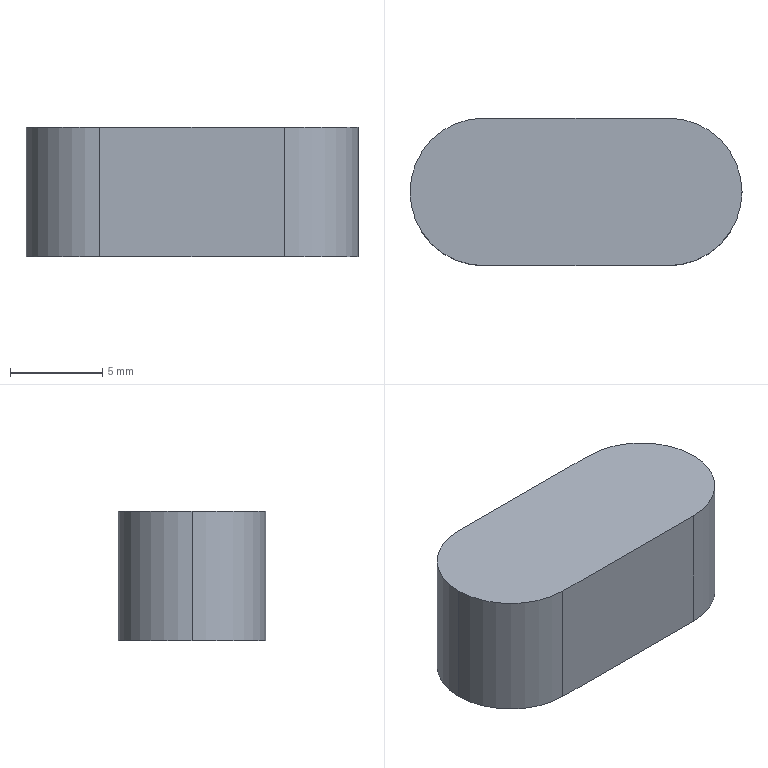Part | SolidWorks | features MBimport 1 | 1 solid | 7 faces | box 18 x 8 x 7 mm | volume 911.858 mm3 | plane 4 | cylinder 3 | commonest cylinder face diameters 8 x3
STEP:
#1=CARTESIAN_POINT('',(-5.,4.,0.));
#2=VERTEX_POINT('',#1);
#3=CARTESIAN_POINT('',(-9.,0.,0.));
#4=VERTEX_POINT('',#3);
#5=CARTESIAN_POINT('',(-5.,0.,0.));
#6=DIRECTION('',(0.,0.,1.));
#7=DIRECTION('',(1.,0.,0.));
#8=AXIS2_PLACEMENT_3D('',#5,#6,#7);
#9=CIRCLE('',#8,4.);
#10=EDGE_CURVE('',#2,#4,#9,.T.);
#11=ORIENTED_EDGE('',*,*,#10,.T.);
#12=CARTESIAN_POINT('',(-9.,0.,7.));
#13=VERTEX_POINT('',#12);
#14=CARTESIAN_POINT('',(-9.,0.,7.));
#15=DIRECTION('',(0.,0.,1.));
#16=VECTOR('',#15,1000.);
#17=LINE('',#14,#16);
#18=EDGE_CURVE('',#4,#13,#17,.T.);
#19=ORIENTED_EDGE('',*,*,#18,.T.);
#20=CARTESIAN_POINT('',(-5.,4.,7.));
#21=VERTEX_POINT('',#20);
#22=CARTESIAN_POINT('',(-5.,0.,7.));
#23=DIRECTION('',(0.,0.,1.));
#24=DIRECTION('',(1.,0.,0.));
#25=AXIS2_PLACEMENT_3D('',#22,#23,#24);
#26=CIRCLE('',#25,4.);
#27=EDGE_CURVE('',#21,#13,#26,.T.);
#28=ORIENTED_EDGE('',*,*,#27,.F.);
#29=CARTESIAN_POINT('',(-5.,4.,7.));
#30=DIRECTION('',(0.,0.,-1.));
#31=VECTOR('',#30,1000.);
#32=LINE('',#29,#31);
#33=EDGE_CURVE('',#21,#2,#32,.T.);
#34=ORIENTED_EDGE('',*,*,#33,.T.);
#35=EDGE_LOOP('',(#11,#19,#28,#34));
#36=FACE_OUTER_BOUND('',#35,.T.);
#37=CARTESIAN_POINT('',(-5.,0.,7.));
#38=DIRECTION('',(0.,0.,1.));
#39=DIRECTION('',(-1.,0.,0.));
#40=AXIS2_PLACEMENT_3D('',#37,#38,#39);
#41=CYLINDRICAL_SURFACE('',#40,4.);
#42=ADVANCED_FACE('',(#36),#41,.T.);
#43=CARTESIAN_POINT('',(5.,4.,0.));
#44=VERTEX_POINT('',#43);
#45=CARTESIAN_POINT('',(5.,4.,0.));
#46=DIRECTION('',(-1.,0.,0.));
#47=VECTOR('',#46,1000.);
#48=LINE('',#45,#47);
#49=EDGE_CURVE('',#44,#2,#48,.T.);
#50=ORIENTED_EDGE('',*,*,#49,.T.);
#51=ORIENTED_EDGE('',*,*,#33,.F.);
#52=CARTESIAN_POINT('',(5.,4.,7.));
#53=VERTEX_POINT('',#52);
#54=CARTESIAN_POINT('',(5.,4.,7.));
#55=DIRECTION('',(-1.,0.,0.));
#56=VECTOR('',#55,1000.);
#57=LINE('',#54,#56);
#58=EDGE_CURVE('',#53,#21,#57,.T.);
#59=ORIENTED_EDGE('',*,*,#58,.F.);
#60=CARTESIAN_POINT('',(5.,4.,7.));
#61=DIRECTION('',(0.,0.,-1.));
#62=VECTOR('',#61,1000.);
#63=LINE('',#60,#62);
#64=EDGE_CURVE('',#53,#44,#63,.T.);
#65=ORIENTED_EDGE('',*,*,#64,.T.);
#66=EDGE_LOOP('',(#50,#51,#59,#65));
#67=FACE_OUTER_BOUND('',#66,.T.);
#68=CARTESIAN_POINT('',(5.,4.,7.));
#69=DIRECTION('',(0.,-1.,0.));
#70=DIRECTION('',(0.,0.,-1.));
#71=AXIS2_PLACEMENT_3D('',#68,#69,#70);
#72=PLANE('',#71);
#73=ADVANCED_FACE('',(#67),#72,.F.);
#74=ORIENTED_EDGE('',*,*,#18,.F.);
#75=CARTESIAN_POINT('',(-5.,-4.,0.));
#76=VERTEX_POINT('',#75);
#77=CARTESIAN_POINT('',(-5.,0.,0.));
#78=DIRECTION('',(0.,0.,1.));
#79=DIRECTION('',(1.,0.,0.));
#80=AXIS2_PLACEMENT_3D('',#77,#78,#79);
#81=CIRCLE('',#80,4.);
#82=EDGE_CURVE('',#4,#76,#81,.T.);
#83=ORIENTED_EDGE('',*,*,#82,.T.);
#84=CARTESIAN_POINT('',(-5.,-4.,7.));
#85=VERTEX_POINT('',#84);
#86=CARTESIAN_POINT('',(-5.,-4.,7.));
#87=DIRECTION('',(0.,0.,-1.));
#88=VECTOR('',#87,1000.);
#89=LINE('',#86,#88);
#90=EDGE_CURVE('',#85,#76,#89,.T.);
#91=ORIENTED_EDGE('',*,*,#90,.F.);
#92=CARTESIAN_POINT('',(-5.,0.,7.));
#93=DIRECTION('',(0.,0.,1.));
#94=DIRECTION('',(1.,0.,0.));
#95=AXIS2_PLACEMENT_3D('',#92,#93,#94);
#96=CIRCLE('',#95,4.);
#97=EDGE_CURVE('',#13,#85,#96,.T.);
#98=ORIENTED_EDGE('',*,*,#97,.F.);
#99=EDGE_LOOP('',(#74,#83,#91,#98));
#100=FACE_OUTER_BOUND('',#99,.T.);
#101=CARTESIAN_POINT('',(-5.,0.,7.));
#102=DIRECTION('',(0.,0.,1.));
#103=DIRECTION('',(-1.,0.,0.));
#104=AXIS2_PLACEMENT_3D('',#101,#102,#103);
#105=CYLINDRICAL_SURFACE('',#104,4.);
#106=ADVANCED_FACE('',(#100),#105,.T.);
#107=CARTESIAN_POINT('',(5.,-4.,0.));
#108=VERTEX_POINT('',#107);
#109=CARTESIAN_POINT('',(-5.,-4.,0.));
#110=DIRECTION('',(1.,0.,0.));
#111=VECTOR('',#110,1000.);
#112=LINE('',#109,#111);
#113=EDGE_CURVE('',#76,#108,#112,.T.);
#114=ORIENTED_EDGE('',*,*,#113,.T.);
#115=CARTESIAN_POINT('',(5.,-4.,7.));
#116=VERTEX_POINT('',#115);
#117=CARTESIAN_POINT('',(5.,-4.,7.));
#118=DIRECTION('',(0.,0.,-1.));
#119=VECTOR('',#118,1000.);
#120=LINE('',#117,#119);
#121=EDGE_CURVE('',#116,#108,#120,.T.);
#122=ORIENTED_EDGE('',*,*,#121,.F.);
#123=CARTESIAN_POINT('',(-5.,-4.,7.));
#124=DIRECTION('',(1.,0.,0.));
#125=VECTOR('',#124,1000.);
#126=LINE('',#123,#125);
#127=EDGE_CURVE('',#85,#116,#126,.T.);
#128=ORIENTED_EDGE('',*,*,#127,.F.);
#129=ORIENTED_EDGE('',*,*,#90,.T.);
#130=EDGE_LOOP('',(#114,#122,#128,#129));
#131=FACE_OUTER_BOUND('',#130,.T.);
#132=CARTESIAN_POINT('',(-5.,-4.,7.));
#133=DIRECTION('',(0.,1.,0.));
#134=DIRECTION('',(1.,0.,0.));
#135=AXIS2_PLACEMENT_3D('',#132,#133,#134);
#136=PLANE('',#135);
#137=ADVANCED_FACE('',(#131),#136,.F.);
#138=CARTESIAN_POINT('',(5.,0.,0.));
#139=DIRECTION('',(0.,0.,1.));
#140=DIRECTION('',(1.,0.,0.));
#141=AXIS2_PLACEMENT_3D('',#138,#139,#140);
#142=CIRCLE('',#141,4.);
#143=EDGE_CURVE('',#108,#44,#142,.T.);
#144=ORIENTED_EDGE('',*,*,#143,.T.);
#145=ORIENTED_EDGE('',*,*,#64,.F.);
#146=CARTESIAN_POINT('',(5.,0.,7.));
#147=DIRECTION('',(0.,0.,1.));
#148=DIRECTION('',(1.,0.,0.));
#149=AXIS2_PLACEMENT_3D('',#146,#147,#148);
#150=CIRCLE('',#149,4.);
#151=EDGE_CURVE('',#116,#53,#150,.T.);
#152=ORIENTED_EDGE('',*,*,#151,.F.);
#153=ORIENTED_EDGE('',*,*,#121,.T.);
#154=EDGE_LOOP('',(#144,#145,#152,#153));
#155=FACE_OUTER_BOUND('',#154,.T.);
#156=CARTESIAN_POINT('',(5.,0.,7.));
#157=DIRECTION('',(0.,0.,1.));
#158=DIRECTION('',(-1.,0.,0.));
#159=AXIS2_PLACEMENT_3D('',#156,#157,#158);
#160=CYLINDRICAL_SURFACE('',#159,4.);
#161=ADVANCED_FACE('',(#155),#160,.T.);
#162=ORIENTED_EDGE('',*,*,#49,.F.);
#163=ORIENTED_EDGE('',*,*,#143,.F.);
#164=ORIENTED_EDGE('',*,*,#113,.F.);
#165=ORIENTED_EDGE('',*,*,#82,.F.);
#166=ORIENTED_EDGE('',*,*,#10,.F.);
#167=EDGE_LOOP('',(#162,#163,#164,#165,#166));
#168=FACE_OUTER_BOUND('',#167,.T.);
#169=CARTESIAN_POINT('',(-5.,0.,0.));
#170=DIRECTION('',(0.,0.,1.));
#171=DIRECTION('',(1.,0.,0.));
#172=AXIS2_PLACEMENT_3D('',#169,#170,#171);
#173=PLANE('',#172);
#174=ADVANCED_FACE('',(#168),#173,.F.);
#175=ORIENTED_EDGE('',*,*,#58,.T.);
#176=ORIENTED_EDGE('',*,*,#27,.T.);
#177=ORIENTED_EDGE('',*,*,#97,.T.);
#178=ORIENTED_EDGE('',*,*,#127,.T.);
#179=ORIENTED_EDGE('',*,*,#151,.T.);
#180=EDGE_LOOP('',(#175,#176,#177,#178,#179));
#181=FACE_OUTER_BOUND('',#180,.T.);
#182=CARTESIAN_POINT('',(-5.,0.,7.));
#183=DIRECTION('',(0.,0.,1.));
#184=DIRECTION('',(1.,0.,0.));
#185=AXIS2_PLACEMENT_3D('',#182,#183,#184);
#186=PLANE('',#185);
#187=ADVANCED_FACE('',(#181),#186,.T.);
#188=CLOSED_SHELL('',(#42,#73,#106,#137,#161,#174,#187));
#189=MANIFOLD_SOLID_BREP('',#188);
#190=CARTESIAN_POINT('',(0.,0.,0.));
#191=DIRECTION('',(0.,0.,1.));
#192=DIRECTION('',(1.,0.,0.));
#193=AXIS2_PLACEMENT_3D('',#190,#191,#192);
#194=(LENGTH_UNIT()NAMED_UNIT(*)SI_UNIT(.MILLI.,.METRE.));
#195=UNCERTAINTY_MEASURE_WITH_UNIT(LENGTH_MEASURE(0.00001),#194,'','');
#196=(NAMED_UNIT(*)PLANE_ANGLE_UNIT()SI_UNIT($,.RADIAN.));
#197=(NAMED_UNIT(*)SI_UNIT($,.STERADIAN.)SOLID_ANGLE_UNIT());
#198=(GEOMETRIC_REPRESENTATION_CONTEXT(3)GLOBAL_UNCERTAINTY_ASSIGNED_CONTEXT((#195))GLOBAL_UNIT_ASSIGNED_CONTEXT((#194,#196,#197))REPRESENTATION_CONTEXT('',''));
#199=ADVANCED_BREP_SHAPE_REPRESENTATION('',(#189,#193),#198);